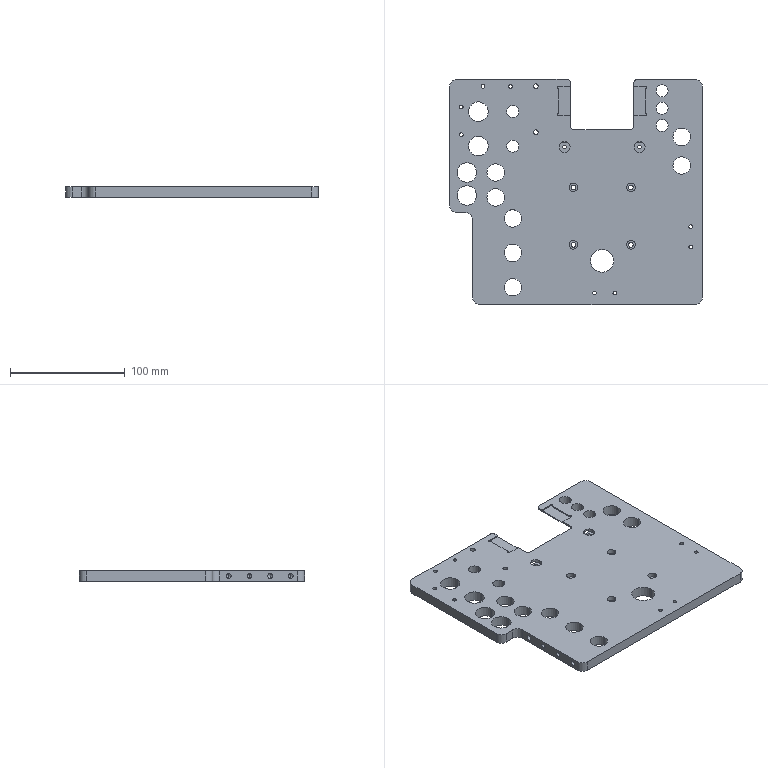NC program | NX | posted with a generic post | part box 220 x 196 x 9 mm
Whole program:
N10 G17 G21 G94 G90
(FLOOR_WALL_COPY_1 , TOOL : D6)
N12 T12 M6
N14 G54
N16 G17 G0 G90 X0.8 Y70.544 S9500 M3
N18 G43 Z30. H12
N20 Z-0.487
N22 G94 G1 X4.5 Y72.68 F2200.
N24 G3 X4.8 Y73.2 R0.6
N26 G1 Y95.
N28 G2 X7.8 Y98. R3.
N30 G1 X21.458
N32 G3 X19.2 Y92. R9.1
N34 G1 Y49.
N36 G2 X16.3 Y46.1 R2.9
N38 G1 X-61.7
N40 G2 X-64.6 Y49. R2.9
N42 G1 Y92.
N44 G3 X-66.858 Y98. R9.1
N46 G1 X-53.25
N48 G2 X-50.25 Y95. R3.
N50 G1 Y54.4
N52 X4.8
N54 Y73.2
N56 X7.8
N58 Y95.
N60 X16.578
N62 G3 X16.2 Y92. R12.1
N64 G1 Y49.1
N66 X-61.6
N68 Y92.
N70 G3 X-61.978 Y95. R12.1
N72 G1 X-53.25
N74 Y54.4
N76 G3 X-53.021 Y53.25 R3.
N78 G1 X-55.792 Y52.1
N80 X-58.6
N82 Y92.
N84 X-56.25
N86 Y54.4
N88 G3 X-55.792 Y52.1 R6.
N90 G1 X-53.021 Y53.25
N92 G3 X-50.25 Y51.4 R3.
N94 G1 X4.8
N96 G3 X7.8 Y54.4 R3.
N98 G1 Y73.2
N100 X10.8
N102 Y92.
N104 X13.2
N106 Y52.1
N108 X10.342
N110 G3 X10.8 Y54.4 R6.
N112 G1 Y73.2
N114 G3 X10.5 Y73.72 R0.6
N116 G0 Z30.
N118 X0.8 Y70.544
N120 Z-0.973
N122 G1 X4.5 Y72.68
N124 G3 X4.8 Y73.2 R0.6
N126 G1 Y95.
N128 G2 X7.8 Y98. R3.
N130 G1 X21.458
N132 G3 X19.2 Y92. R9.1
N134 G1 Y49.
N136 G2 X16.3 Y46.1 R2.9
N138 G1 X-61.7
N140 G2 X-64.6 Y49. R2.9
N142 G1 Y92.
N144 G3 X-66.858 Y98. R9.1
N146 G1 X-53.25
N148 G2 X-50.25 Y95. R3.
N150 G1 Y54.4
N152 X4.8
N154 Y73.2
N156 X7.8
N158 Y95.
N160 X16.578
N162 G3 X16.2 Y92. R12.1
N164 G1 Y49.1
N166 X-61.6
N168 Y92.
N170 G3 X-61.978 Y95. R12.1
N172 G1 X-53.25
N174 Y54.4
N176 G3 X-53.021 Y53.25 R3.
N178 G1 X-55.792 Y52.1
N180 X-58.6
N182 Y92.
N184 X-56.25
N186 Y54.4
N188 G3 X-55.792 Y52.1 R6.
N190 G1 X-53.021 Y53.25
N192 G3 X-50.25 Y51.4 R3.
N194 G1 X4.8
N196 G3 X7.8 Y54.4 R3.
N198 G1 Y73.2
N200 X10.8
N202 Y92.
N204 X13.2
N206 Y52.1
N208 X10.342
N210 G3 X10.8 Y54.4 R6.
N212 G1 Y73.2
N214 G3 X10.5 Y73.72 R0.6
N216 G0 Z30.
N218 X0.8 Y70.544
N220 Z-1.46
N222 G1 X4.5 Y72.68
N224 G3 X4.8 Y73.2 R0.6
N226 G1 Y95.
N228 G2 X7.8 Y98. R3.
N230 G1 X21.458
N232 G3 X19.2 Y92. R9.1
N234 G1 Y49.
N236 G2 X16.3 Y46.1 R2.9
N238 G1 X-61.7
N240 G2 X-64.6 Y49. R2.9
N242 G1 Y92.
N244 G3 X-66.858 Y98. R9.1
N246 G1 X-53.25
N248 G2 X-50.25 Y95. R3.
N250 G1 Y54.4
N252 X4.8
N254 Y73.2
N256 X7.8
N258 Y95.
N260 X16.578
N262 G3 X16.2 Y92. R12.1
N264 G1 Y49.1
N266 X-61.6
N268 Y92.
N270 G3 X-61.978 Y95. R12.1
N272 G1 X-53.25
N274 Y54.4
N276 G3 X-53.021 Y53.25 R3.
N278 G1 X-55.792 Y52.1
N280 X-58.6
N282 Y92.
N284 X-56.25
N286 Y54.4
N288 G3 X-55.792 Y52.1 R6.
N290 G1 X-53.021 Y53.25
N292 G3 X-50.25 Y51.4 R3.
N294 G1 X4.8
N296 G3 X7.8 Y54.4 R3.
N298 G1 Y73.2
N300 X10.8
N302 Y92.
N304 X13.2
N306 Y52.1
N308 X10.342
N310 G3 X10.8 Y54.4 R6.
N312 G1 Y73.2
N314 G3 X10.5 Y73.72 R0.6
N316 G0 Z30.
N318 X0.8 Y70.544
N320 Z-1.947
N322 G1 X4.5 Y72.68
N324 G3 X4.8 Y73.2 R0.6
N326 G1 Y95.
N328 G2 X7.8 Y98. R3.
N330 G1 X21.458
N332 G3 X19.2 Y92. R9.1
N334 G1 Y49.
N336 G2 X16.3 Y46.1 R2.9
N338 G1 X-61.7
N340 G2 X-64.6 Y49. R2.9
N342 G1 Y92.
N344 G3 X-66.858 Y98. R9.1
N346 G1 X-53.25
N348 G2 X-50.25 Y95. R3.
N350 G1 Y54.4
N352 X4.8
N354 Y73.2
N356 X7.8
N358 Y95.
N360 X16.578
N362 G3 X16.2 Y92. R12.1
N364 G1 Y49.1
N366 X-61.6
N368 Y92.
N370 G3 X-61.978 Y95. R12.1
N372 G1 X-53.25
N374 Y54.4
N376 G3 X-53.021 Y53.25 R3.
N378 G1 X-55.792 Y52.1
N380 X-58.6
N382 Y92.
N384 X-56.25
N386 Y54.4
N388 G3 X-55.792 Y52.1 R6.
N390 G1 X-53.021 Y53.25
N392 G3 X-50.25 Y51.4 R3.
N394 G1 X4.8
N396 G3 X7.8 Y54.4 R3.
N398 G1 Y73.2
N400 X10.8
N402 Y92.
N404 X13.2
N406 Y52.1
N408 X10.342
N410 G3 X10.8 Y54.4 R6.
N412 G1 Y73.2
N414 G3 X10.5 Y73.72 R0.6
N416 G0 Z30.
N418 X0.8 Y70.544
N420 Z-2.433
N422 G1 X4.5 Y72.68
N424 G3 X4.8 Y73.2 R0.6
N426 G1 Y95.
N428 G2 X7.8 Y98. R3.
N430 G1 X21.458
N432 G3 X19.2 Y92. R9.1
N434 G1 Y49.
N436 G2 X16.3 Y46.1 R2.9
N438 G1 X-61.7
N440 G2 X-64.6 Y49. R2.9
N442 G1 Y92.
N444 G3 X-66.858 Y98. R9.1
N446 G1 X-53.25
N448 G2 X-50.25 Y95. R3.
N450 G1 Y54.4
N452 X4.8
N454 Y73.2
N456 X7.8
N458 Y95.
N460 X16.578
N462 G3 X16.2 Y92. R12.1
N464 G1 Y49.1
N466 X-61.6
N468 Y92.
N470 G3 X-61.978 Y95. R12.1
N472 G1 X-53.25
N474 Y54.4
N476 G3 X-53.021 Y53.25 R3.
N478 G1 X-55.792 Y52.1
N480 X-58.6
N482 Y92.
N484 X-56.25
N486 Y54.4
N488 G3 X-55.792 Y52.1 R6.
N490 G1 X-53.021 Y53.25
N492 G3 X-50.25 Y51.4 R3.
N494 G1 X4.8
N496 G3 X7.8 Y54.4 R3.
N498 G1 Y73.2
N500 X10.8
N502 Y92.
N504 X13.2
N506 Y52.1
N508 X10.342
N510 G3 X10.8 Y54.4 R6.
N512 G1 Y73.2
N514 G3 X10.5 Y73.72 R0.6
N516 G0 Z30.
N518 X0.8 Y70.544
N520 Z-2.92
N522 G1 X4.5 Y72.68
N524 G3 X4.8 Y73.2 R0.6
N526 G1 Y95.
N528 G2 X7.8 Y98. R3.
N530 G1 X21.458
N532 G3 X19.2 Y92. R9.1
N534 G1 Y49.
N536 G2 X16.3 Y46.1 R2.9
N538 G1 X-61.7
N540 G2 X-64.6 Y49. R2.9
N542 G1 Y92.
N544 G3 X-66.858 Y98. R9.1
N546 G1 X-53.25
N548 G2 X-50.25 Y95. R3.
N550 G1 Y54.4
N552 X4.8
N554 Y73.2
N556 X7.8
N558 Y95.
N560 X16.578
N562 G3 X16.2 Y92. R12.1
N564 G1 Y49.1
N566 X-61.6
N568 Y92.
N570 G3 X-61.978 Y95. R12.1
N572 G1 X-53.25
N574 Y54.4
N576 G3 X-53.021 Y53.25 R3.
N578 G1 X-55.792 Y52.1
N580 X-58.6
N582 Y92.
N584 X-56.25
N586 Y54.4
N588 G3 X-55.792 Y52.1 R6.
N590 G1 X-53.021 Y53.25
N592 G3 X-50.25 Y51.4 R3.
N594 G1 X4.8
N596 G3 X7.8 Y54.4 R3.
N598 G1 Y73.2
N600 X10.8
N602 Y92.
N604 X13.2
N606 Y52.1
N608 X10.342
N610 G3 X10.8 Y54.4 R6.
N612 G1 Y73.2
N614 G3 X10.5 Y73.72 R0.6
N616 G0 Z30.
N618 X0.8 Y70.544
N620 Z-3.407
N622 G1 X4.5 Y72.68
N624 G3 X4.8 Y73.2 R0.6
N626 G1 Y95.
N628 G2 X7.8 Y98. R3.
N630 G1 X21.458
N632 G3 X19.2 Y92. R9.1
N634 G1 Y49.
N636 G2 X16.3 Y46.1 R2.9
N638 G1 X-61.7
N640 G2 X-64.6 Y49. R2.9
N642 G1 Y92.
N644 G3 X-66.858 Y98. R9.1
N646 G1 X-53.25
N648 G2 X-50.25 Y95. R3.
N650 G1 Y54.4
N652 X4.8
N654 Y73.2
N656 X7.8
N658 Y95.
N660 X16.578
N662 G3 X16.2 Y92. R12.1
N664 G1 Y49.1
N666 X-61.6
N668 Y92.
N670 G3 X-61.978 Y95. R12.1
N672 G1 X-53.25
N674 Y54.4
N676 G3 X-53.021 Y53.25 R3.
N678 G1 X-55.792 Y52.1
N680 X-58.6
N682 Y92.
N684 X-56.25
N686 Y54.4
N688 G3 X-55.792 Y52.1 R6.
N690 G1 X-53.021 Y53.25
N692 G3 X-50.25 Y51.4 R3.
N694 G1 X4.8
N696 G3 X7.8 Y54.4 R3.
N698 G1 Y73.2
N700 X10.8
N702 Y92.
N704 X13.2
N706 Y52.1
N708 X10.342
N710 G3 X10.8 Y54.4 R6.
N712 G1 Y73.2
N714 G3 X10.5 Y73.72 R0.6
N716 G0 Z30.
N718 X0.8 Y70.544
N720 Z-3.893
N722 G1 X4.5 Y72.68
N724 G3 X4.8 Y73.2 R0.6
N726 G1 Y95.
N728 G2 X7.8 Y98. R3.
N730 G1 X21.458
N732 G3 X19.2 Y92. R9.1
N734 G1 Y49.
N736 G2 X16.3 Y46.1 R2.9
N738 G1 X-61.7
N740 G2 X-64.6 Y49. R2.9
N742 G1 Y92.
N744 G3 X-66.858 Y98. R9.1
N746 G1 X-53.25
N748 G2 X-50.25 Y95. R3.
N750 G1 Y54.4
N752 X4.8
N754 Y73.2
N756 X7.8
N758 Y95.
N760 X16.578
N762 G3 X16.2 Y92. R12.1
N764 G1 Y49.1
N766 X-61.6
N768 Y92.
N770 G3 X-61.978 Y95. R12.1
N772 G1 X-53.25
N774 Y54.4
N776 G3 X-53.021 Y53.25 R3.
N778 G1 X-55.792 Y52.1
N780 X-58.6
N782 Y92.
N784 X-56.25
N786 Y54.4
N788 G3 X-55.792 Y52.1 R6.
N790 G1 X-53.021 Y53.25
N792 G3 X-50.25 Y51.4 R3.
N794 G1 X4.8
N796 G3 X7.8 Y54.4 R3.
N798 G1 Y73.2
N800 X10.8
N802 Y92.
N804 X13.2
N806 Y52.1
N808 X10.342
N810 G3 X10.8 Y54.4 R6.
N812 G1 Y73.2
N814 G3 X10.5 Y73.72 R0.6
N816 G0 Z30.
N818 X0.8 Y70.544
N820 Z-4.38
N822 G1 X4.5 Y72.68
N824 G3 X4.8 Y73.2 R0.6
N826 G1 Y95.
N828 G2 X7.8 Y98. R3.
N830 G1 X21.458
N832 G3 X19.2 Y92. R9.1
N834 G1 Y49.
N836 G2 X16.3 Y46.1 R2.9
N838 G1 X-61.7
N840 G2 X-64.6 Y49. R2.9
N842 G1 Y92.
N844 G3 X-66.858 Y98. R9.1
N846 G1 X-53.25
N848 G2 X-50.25 Y95. R3.
N850 G1 Y54.4
N852 X4.8
N854 Y73.2
N856 X7.8
N858 Y95.
N860 X16.578
N862 G3 X16.2 Y92. R12.1
N864 G1 Y49.1
N866 X-61.6
N868 Y92.
N870 G3 X-61.978 Y95. R12.1
N872 G1 X-53.25
N874 Y54.4
N876 G3 X-53.021 Y53.25 R3.
N878 G1 X-55.792 Y52.1
N880 X-58.6
N882 Y92.
N884 X-56.25
N886 Y54.4
N888 G3 X-55.792 Y52.1 R6.
N890 G1 X-53.021 Y53.25
N892 G3 X-50.25 Y51.4 R3.
N894 G1 X4.8
N896 G3 X7.8 Y54.4 R3.
N898 G1 Y73.2
N900 X10.8
N902 Y92.
N904 X13.2
N906 Y52.1
N908 X10.342
N910 G3 X10.8 Y54.4 R6.
N912 G1 Y73.2
N914 G3 X10.5 Y73.72 R0.6
N916 G0 Z30.
N918 X0.8 Y70.544
N920 Z-4.867
N922 G1 X4.5 Y72.68
N924 G3 X4.8 Y73.2 R0.6
N926 G1 Y95.
N928 G2 X7.8 Y98. R3.
N930 G1 X21.458
N932 G3 X19.2 Y92. R9.1
N934 G1 Y49.
N936 G2 X16.3 Y46.1 R2.9
N938 G1 X-61.7
N940 G2 X-64.6 Y49. R2.9
N942 G1 Y92.
N944 G3 X-66.858 Y98. R9.1
N946 G1 X-53.25
N948 G2 X-50.25 Y95. R3.
N950 G1 Y54.4
N952 X4.8
N954 Y73.2
N956 X7.8
N958 Y95.
N960 X16.578
N962 G3 X16.2 Y92. R12.1
N964 G1 Y49.1
N966 X-61.6
N968 Y92.
N970 G3 X-61.978 Y95. R12.1
N972 G1 X-53.25
N974 Y54.4
N976 G3 X-53.021 Y53.25 R3.
N978 G1 X-55.792 Y52.1
N980 X-58.6
N982 Y92.
N984 X-56.25
N986 Y54.4
N988 G3 X-55.792 Y52.1 R6.
N990 G1 X-53.021 Y53.25
N992 G3 X-50.25 Y51.4 R3.
N994 G1 X4.8
N996 G3 X7.8 Y54.4 R3.
N998 G1 Y73.2
N1000 X10.8
N1002 Y92.
N1004 X13.2
N1006 Y52.1
N1008 X10.342
N1010 G3 X10.8 Y54.4 R6.
N1012 G1 Y73.2
N1014 G3 X10.5 Y73.72 R0.6
N1016 G0 Z30.
N1018 X0.8 Y70.544
N1020 Z-5.353
N1022 G1 X4.5 Y72.68
N1024 G3 X4.8 Y73.2 R0.6
N1026 G1 Y95.
N1028 G2 X7.8 Y98. R3.
N1030 G1 X21.458
N1032 G3 X19.2 Y92. R9.1
N1034 G1 Y49.
N1036 G2 X16.3 Y46.1 R2.9
N1038 G1 X-61.7
N1040 G2 X-64.6 Y49. R2.9
N1042 G1 Y92.
N1044 G3 X-66.858 Y98. R9.1
N1046 G1 X-53.25
N1048 G2 X-50.25 Y95. R3.
N1050 G1 Y54.4
N1052 X4.8
N1054 Y73.2
N1056 X7.8
N1058 Y95.
N1060 X16.578
N1062 G3 X16.2 Y92. R12.1
N1064 G1 Y49.1
N1066 X-61.6
N1068 Y92.
N1070 G3 X-61.978 Y95. R12.1
N1072 G1 X-53.25
N1074 Y54.4
N1076 G3 X-53.021 Y53.25 R3.
N1078 G1 X-55.792 Y52.1
N1080 X-58.6
N1082 Y92.
N1084 X-56.25
N1086 Y54.4
N1088 G3 X-55.792 Y52.1 R6.
N1090 G1 X-53.021 Y53.25
N1092 G3 X-50.25 Y51.4 R3.
N1094 G1 X4.8
N1096 G3 X7.8 Y54.4 R3.
N1098 G1 Y73.2
N1100 X10.8
N1102 Y92.
N1104 X13.2
N1106 Y52.1
N1108 X10.342
N1110 G3 X10.8 Y54.4 R6.
N1112 G1 Y73.2
N1114 G3 X10.5 Y73.72 R0.6
N1116 G0 Z30.
N1118 X0.8 Y70.544
N1120 Z-5.84
N1122 G1 X4.5 Y72.68
N1124 G3 X4.8 Y73.2 R0.6
N1126 G1 Y95.
N1128 G2 X7.8 Y98. R3.
N1130 G1 X21.458
N1132 G3 X19.2 Y92. R9.1
N1134 G1 Y49.
N1136 G2 X16.3 Y46.1 R2.9
N1138 G1 X-61.7
N1140 G2 X-64.6 Y49. R2.9
N1142 G1 Y92.
N1144 G3 X-66.858 Y98. R9.1
N1146 G1 X-53.25
N1148 G2 X-50.25 Y95. R3.
N1150 G1 Y54.4
N1152 X4.8
N1154 Y73.2
N1156 X7.8
N1158 Y95.
N1160 X16.578
N1162 G3 X16.2 Y92. R12.1
N1164 G1 Y49.1
N1166 X-61.6
N1168 Y92.
N1170 G3 X-61.978 Y95. R12.1
N1172 G1 X-53.25
N1174 Y54.4
N1176 G3 X-53.021 Y53.25 R3.
N1178 G1 X-55.792 Y52.1
N1180 X-58.6
N1182 Y92.
N1184 X-56.25
N1186 Y54.4
N1188 G3 X-55.792 Y52.1 R6.
N1190 G1 X-53.021 Y53.25
N1192 G3 X-50.25 Y51.4 R3.
N1194 G1 X4.8
N1196 G3 X7.8 Y54.4 R3.
N1198 G1 Y73.2
N1200 X10.8
N1202 Y92.
N1204 X13.2
N1206 Y52.1
N1208 X10.342
N1210 G3 X10.8 Y54.4 R6.
N1212 G1 Y73.2
N1214 G3 X10.5 Y73.72 R0.6
N1216 G0 Z30.
N1218 X0.8 Y70.544
N1220 Z-6.327
N1222 G1 X4.5 Y72.68
N1224 G3 X4.8 Y73.2 R0.6
N1226 G1 Y95.
N1228 G2 X7.8 Y98. R3.
N1230 G1 X21.458
N1232 G3 X19.2 Y92. R9.1
N1234 G1 Y49.
N1236 G2 X16.3 Y46.1 R2.9
N1238 G1 X-61.7
N1240 G2 X-64.6 Y49. R2.9
N1242 G1 Y92.
N1244 G3 X-66.858 Y98. R9.1
N1246 G1 X-53.25
N1248 G2 X-50.25 Y95. R3.
N1250 G1 Y54.4
N1252 X4.8
N1254 Y73.2
N1256 X7.8
N1258 Y95.
N1260 X16.578
N1262 G3 X16.2 Y92. R12.1
N1264 G1 Y49.1
N1266 X-61.6
N1268 Y92.
N1270 G3 X-61.978 Y95. R12.1
N1272 G1 X-53.25
N1274 Y54.4
N1276 G3 X-53.021 Y53.25 R3.
N1278 G1 X-55.792 Y52.1
N1280 X-58.6
N1282 Y92.
N1284 X-56.25
N1286 Y54.4
N1288 G3 X-55.792 Y52.1 R6.
N1290 G1 X-53.021 Y53.25
N1292 G3 X-50.25 Y51.4 R3.
N1294 G1 X4.8
N1296 G3 X7.8 Y54.4 R3.
N1298 G1 Y73.2
N1300 X10.8
N1302 Y92.
N1304 X13.2
N1306 Y52.1
N1308 X10.342
N1310 G3 X10.8 Y54.4 R6.
N1312 G1 Y73.2
N1314 G3 X10.5 Y73.72 R0.6
N1316 G0 Z30.
N1318 X0.8 Y70.544
N1320 Z-6.813
N1322 G1 X4.5 Y72.68
N1324 G3 X4.8 Y73.2 R0.6
N1326 G1 Y95.
N1328 G2 X7.8 Y98. R3.
N1330 G1 X21.458
N1332 G3 X19.2 Y92. R9.1
N1334 G1 Y49.
N1336 G2 X16.3 Y46.1 R2.9
N1338 G1 X-61.7
N1340 G2 X-64.6 Y49. R2.9
N1342 G1 Y92.
N1344 G3 X-66.858 Y98. R9.1
N1346 G1 X-53.25
N1348 G2 X-50.25 Y95. R3.
N1350 G1 Y54.4
N1352 X4.8
N1354 Y73.2
N1356 X7.8
N1358 Y95.
N1360 X16.578
N1362 G3 X16.2 Y92. R12.1
N1364 G1 Y49.1
N1366 X-61.6
N1368 Y92.
N1370 G3 X-61.978 Y95. R12.1
N1372 G1 X-53.25
N1374 Y54.4
N1376 G3 X-53.021 Y53.25 R3.
N1378 G1 X-55.792 Y52.1
N1380 X-58.6
N1382 Y92.
N1384 X-56.25
N1386 Y54.4
N1388 G3 X-55.792 Y52.1 R6.
N1390 G1 X-53.021 Y53.25
N1392 G3 X-50.25 Y51.4 R3.
N1394 G1 X4.8
N1396 G3 X7.8 Y54.4 R3.
N1398 G1 Y73.2
N1400 X10.8
N1402 Y92.
N1404 X13.2
N1406 Y52.1
N1408 X10.342
N1410 G3 X10.8 Y54.4 R6.
N1412 G1 Y73.2
N1414 G3 X10.5 Y73.72 R0.6
N1416 G0 Z30.
N1418 X0.8 Y70.544
N1420 Z-7.3
N1422 G1 X4.5 Y72.68
N1424 G3 X4.8 Y73.2 R0.6
N1426 G1 Y95.
N1428 G2 X7.8 Y98. R3.
N1430 G1 X21.458
N1432 G3 X19.2 Y92. R9.1
N1434 G1 Y49.
N1436 G2 X16.3 Y46.1 R2.9
N1438 G1 X-61.7
N1440 G2 X-64.6 Y49. R2.9
N1442 G1 Y92.
N1444 G3 X-66.858 Y98. R9.1
N1446 G1 X-53.25
N1448 G2 X-50.25 Y95. R3.
N1450 G1 Y54.4
N1452 X4.8
N1454 Y73.2
N1456 X7.8
N1458 Y95.
N1460 X16.578
N1462 G3 X16.2 Y92. R12.1
N1464 G1 Y49.1
N1466 X-61.6
N1468 Y92.
N1470 G3 X-61.978 Y95. R12.1
N1472 G1 X-53.25
N1474 Y54.4
N1476 G3 X-53.021 Y53.25 R3.
N1478 G1 X-55.792 Y52.1
N1480 X-58.6
N1482 Y92.
N1484 X-56.25
N1486 Y54.4
N1488 G3 X-55.792 Y52.1 R6.
N1490 G1 X-53.021 Y53.25
N1492 G3 X-50.25 Y51.4 R3.
N1494 G1 X4.8
N1496 G3 X7.8 Y54.4 R3.
N1498 G1 Y73.2
N1500 X10.8
N1502 Y92.
N1504 X13.2
N1506 Y52.1
N1508 X10.342
N1510 G3 X10.8 Y54.4 R6.
N1512 G1 Y73.2
N1514 G3 X10.5 Y73.72 R0.6
N1516 G0 Z30.
(FLOOR_WALL_1 , TOOL : D6)
N1518 X-1.2 Y60.4
N1520 Z-4.4
N1522 G1 Z-7.4 F1250.
N1524 Y57.4
N1526 X1.8
N1528 Y95.
N1530 G2 X7.8 Y101. R6.
N1532 G1 X25.957
N1534 G3 X19. Y92. R9.3
N1536 G1 Y49.
N1538 G2 X16.3 Y46.3 R2.7
N1540 G1 X-61.7
N1542 G2 X-64.4 Y49. R2.7
N1544 G1 Y92.
N1546 G3 X-71.357 Y101. R9.3
N1548 G1 X-53.25
N1550 G2 X-47.25 Y95. R6.
N1552 G1 Y57.4
N1554 X1.8
N1556 X3.745 Y55.116
N1558 G3 X4.8 Y57.4 R3.
N1560 G1 Y95.
N1562 G2 X7.8 Y98. R3.
N1564 G1 X17.563
N1566 G3 X16. Y92. R12.3
N1568 G1 Y49.3
N1570 X-61.4
N1572 Y92.
N1574 G3 X-62.963 Y98. R12.3
N1576 G1 X-53.25
N1578 G2 X-50.25 Y95. R3.
N1580 G1 Y57.4
N1582 G3 X-48.83 Y54.85 R3.
N1584 G1 X-50.411 Y52.3
N1586 X-58.4
N1588 Y92.
N1590 G3 X-58.697 Y95. R15.3
N1592 G1 X-53.25
N1594 Y57.4
N1596 G3 X-50.411 Y52.3 R6.
N1598 G1 X-55.612 Y55.
N1600 X-55.7
N1602 Y55.329
N1604 G3 X-55.612 Y55. R8.7
N1606 G1 X-50.411 Y52.3
N1608 X-48.83 Y54.85
N1610 G3 X-47.25 Y54.4 R3.
N1612 G1 X1.8
N1614 G3 X3.745 Y55.116 R3.
N1616 G1 X5.69 Y52.832
N1618 G3 X7.8 Y57.4 R6.
N1620 G1 Y95.
N1622 X13.297
N1624 G3 X13. Y92. R15.3
N1626 G1 Y52.3
N1628 X4.961
N1630 G3 X5.69 Y52.832 R6.
N1632 G1 X10.162 Y55.
N1634 G3 X10.3 Y55.545 R8.7
N1636 G1 Y55.
N1638 X10.162
N1640 Y52.
N1642 Z-4.4
N1644 G0 Z30.
N1646 X-75.956 Y104.
N1648 Z-4.4
N1650 G1 Z-7.4
N1652 Y101.215
N1654 X-72.966 Y100.97
N1656 G2 X-64.7 Y92. R9.
N1658 G1 Y49.
N1660 G3 X-61.7 Y46. R3.
N1662 G1 X16.3
N1664 G3 X19.3 Y49. R3.
N1666 G1 Y92.
N1668 G2 X27.566 Y100.97 R9.
N1670 G1 X30.556 Y101.215
N1672 Y104.
N1674 Z-4.4
N1676 G0 Z30.
(HOLE_MILLING_COPY , TOOL : D6)
N1678 X35. Y92.
N1680 Z0.5
N1682 G3 X34.625 Y92.375 R0.375
N1684 X34.25 Y92. R0.375
N1686 X34.25 Y92. Z0. I0.75 J0.
N1688 X34.25 Y92. Z-0.5 I0.75 J0.
N1690 X34.25 Y92. Z-1. I0.75 J0.
N1692 X34.25 Y92. Z-1.5 I0.75 J0.
N1694 X34.25 Y92. Z-2. I0.75 J0.
N1696 X34.25 Y92. Z-2.5 I0.75 J0.
N1698 X34.25 Y92. Z-3. I0.75 J0.
N1700 X34.25 Y92. Z-3.5 I0.75 J0.
N1702 X34.25 Y92. Z-4. I0.75 J0.
N1704 X35. Y91.25 R0.75
N1706 X34.25 Y92. R-0.75
N1708 X34.625 Y91.625 R0.375
N1710 X35. Y92. R0.375
N1712 G0 Z30.
N1714 Y52.
N1716 Z0.5
N1718 G3 X34.625 Y52.375 R0.375
N1720 X34.25 Y52. R0.375
N1722 X34.25 Y52. Z0. I0.75 J0.
N1724 X34.25 Y52. Z-0.5 I0.75 J0.
N1726 X34.25 Y52. Z-1. I0.75 J0.
N1728 X34.25 Y52. Z-1.5 I0.75 J0.
N1730 X34.25 Y52. Z-2. I0.75 J0.
N1732 X34.25 Y52. Z-2.5 I0.75 J0.
N1734 X34.25 Y52. Z-3. I0.75 J0.
N1736 X34.25 Y52. Z-3.5 I0.75 J0.
N1738 X34.25 Y52. Z-4. I0.75 J0.
N1740 X35. Y51.25 R0.75
N1742 X34.25 Y52. R-0.75
N1744 X34.625 Y51.625 R0.375
N1746 X35. Y52. R0.375
N1748 G0 Z30.
N1750 M5
(HOLE_MILLING_1 , TOOL : D3)
N1752 T18 M6
N1754 G54
N1756 G17 G0 G90 X-103. Y-68. S9500 M3
N1758 G43 Z30. H18
N1760 Z1.
N1762 G94 G3 X-103.3 Y-67.7 R0.3 F1250.
N1764 X-103.6 Y-68. R0.3
N1766 X-103.6 Y-68. Z0.8 I0.6 J0.
N1768 X-103.6 Y-68. Z0.6 I0.6 J0.
N1770 X-103.6 Y-68. Z0.4 I0.6 J0.
N1772 X-103.6 Y-68. Z0.2 I0.6 J0.
N1774 X-103.6 Y-68. Z0. I0.6 J0.
N1776 X-103.6 Y-68. Z-0.2 I0.6 J0.
N1778 X-103.6 Y-68. Z-0.4 I0.6 J0.
N1780 X-103.6 Y-68. Z-0.6 I0.6 J0.
N1782 X-103.6 Y-68. Z-0.8 I0.6 J0.
N1784 X-103.6 Y-68. Z-1. I0.6 J0.
N1786 X-103.6 Y-68. Z-1.2 I0.6 J0.
N1788 X-103.6 Y-68. Z-1.4 I0.6 J0.
N1790 X-103.6 Y-68. Z-1.6 I0.6 J0.
N1792 X-103.6 Y-68. Z-1.8 I0.6 J0.
N1794 X-103.6 Y-68. Z-2. I0.6 J0.
N1796 X-103.6 Y-68. Z-2.2 I0.6 J0.
N1798 X-103.6 Y-68. Z-2.4 I0.6 J0.
N1800 X-103.6 Y-68. Z-2.6 I0.6 J0.
N1802 X-103.6 Y-68. Z-2.8 I0.6 J0.
N1804 X-103.6 Y-68. Z-3. I0.6 J0.
N1806 X-103.6 Y-68. Z-3.2 I0.6 J0.
N1808 X-103.6 Y-68. Z-3.4 I0.6 J0.
N1810 X-103.6 Y-68. Z-3.6 I0.6 J0.
N1812 X-103.6 Y-68. Z-3.8 I0.6 J0.
N1814 X-103.6 Y-68. Z-4. I0.6 J0.
N1816 X-103.6 Y-68. Z-4.2 I0.6 J0.
N1818 X-103.6 Y-68. Z-4.4 I0.6 J0.
N1820 X-103.6 Y-68. Z-4.6 I0.6 J0.
N1822 X-103.6 Y-68. Z-4.8 I0.6 J0.
N1824 X-103.6 Y-68. Z-5. I0.6 J0.
N1826 X-103.6 Y-68. Z-5.2 I0.6 J0.
N1828 X-103.6 Y-68. Z-5.4 I0.6 J0.
N1830 X-103.6 Y-68. Z-5.6 I0.6 J0.
N1832 X-103.6 Y-68. Z-5.8 I0.6 J0.
N1834 X-103.6 Y-68. Z-6. I0.6 J0.
N1836 X-103. Y-68.6 R0.6
N1838 X-103.6 Y-68. R-0.6
N1840 X-103.3 Y-68.3 R0.3
N1842 X-103. Y-68. R0.3
N1844 G0 Z30.
N1846 Y-86.
N1848 Z1.
N1850 G3 X-103.3 Y-85.7 R0.3
N1852 X-103.6 Y-86. R0.3
N1854 X-103.6 Y-86. Z0.8 I0.6 J0.
N1856 X-103.6 Y-86. Z0.6 I0.6 J0.
N1858 X-103.6 Y-86. Z0.4 I0.6 J0.
N1860 X-103.6 Y-86. Z0.2 I0.6 J0.
N1862 X-103.6 Y-86. Z0. I0.6 J0.
N1864 X-103.6 Y-86. Z-0.2 I0.6 J0.
N1866 X-103.6 Y-86. Z-0.4 I0.6 J0.
N1868 X-103.6 Y-86. Z-0.6 I0.6 J0.
N1870 X-103.6 Y-86. Z-0.8 I0.6 J0.
N1872 X-103.6 Y-86. Z-1. I0.6 J0.
N1874 X-103.6 Y-86. Z-1.2 I0.6 J0.
N1876 X-103.6 Y-86. Z-1.4 I0.6 J0.
N1878 X-103.6 Y-86. Z-1.6 I0.6 J0.
N1880 X-103.6 Y-86. Z-1.8 I0.6 J0.
N1882 X-103.6 Y-86. Z-2. I0.6 J0.
N1884 X-103.6 Y-86. Z-2.2 I0.6 J0.
N1886 X-103.6 Y-86. Z-2.4 I0.6 J0.
N1888 X-103.6 Y-86. Z-2.6 I0.6 J0.
N1890 X-103.6 Y-86. Z-2.8 I0.6 J0.
N1892 X-103.6 Y-86. Z-3. I0.6 J0.
N1894 X-103.6 Y-86. Z-3.2 I0.6 J0.
N1896 X-103.6 Y-86. Z-3.4 I0.6 J0.
N1898 X-103.6 Y-86. Z-3.6 I0.6 J0.
N1900 X-103.6 Y-86. Z-3.8 I0.6 J0.
N1902 X-103.6 Y-86. Z-4. I0.6 J0.
N1904 X-103.6 Y-86. Z-4.2 I0.6 J0.
N1906 X-103.6 Y-86. Z-4.4 I0.6 J0.
N1908 X-103.6 Y-86. Z-4.6 I0.6 J0.
N1910 X-103.6 Y-86. Z-4.8 I0.6 J0.
N1912 X-103.6 Y-86. Z-5. I0.6 J0.
N1914 X-103.6 Y-86. Z-5.2 I0.6 J0.
N1916 X-103.6 Y-86. Z-5.4 I0.6 J0.
N1918 X-103.6 Y-86. Z-5.6 I0.6 J0.
N1920 X-103.6 Y-86. Z-5.8 I0.6 J0.
N1922 X-103.6 Y-86. Z-6. I0.6 J0.
N1924 X-103. Y-86.6 R0.6
N1926 X-103.6 Y-86. R-0.6
N1928 X-103.3 Y-86.3 R0.3
N1930 X-103. Y-86. R0.3
N1932 G0 Z30.
N1934 X83.
N1936 Z1.
N1938 G3 X82.7 Y-85.7 R0.3
N1940 X82.4 Y-86. R0.3
N1942 X82.4 Y-86. Z0.8 I0.6 J0.
N1944 X82.4 Y-86. Z0.6 I0.6 J0.
N1946 X82.4 Y-86. Z0.4 I0.6 J0.
N1948 X82.4 Y-86. Z0.2 I0.6 J0.
N1950 X82.4 Y-86. Z0. I0.6 J0.
N1952 X82.4 Y-86. Z-0.2 I0.6 J0.
N1954 X82.4 Y-86. Z-0.4 I0.6 J0.
N1956 X82.4 Y-86. Z-0.6 I0.6 J0.
N1958 X82.4 Y-86. Z-0.8 I0.6 J0.
N1960 X82.4 Y-86. Z-1. I0.6 J0.
N1962 X82.4 Y-86. Z-1.2 I0.6 J0.
N1964 X82.4 Y-86. Z-1.4 I0.6 J0.
N1966 X82.4 Y-86. Z-1.6 I0.6 J0.
N1968 X82.4 Y-86. Z-1.8 I0.6 J0.
N1970 X82.4 Y-86. Z-2. I0.6 J0.
N1972 X82.4 Y-86. Z-2.2 I0.6 J0.
N1974 X82.4 Y-86. Z-2.4 I0.6 J0.
N1976 X82.4 Y-86. Z-2.6 I0.6 J0.
N1978 X82.4 Y-86. Z-2.8 I0.6 J0.
N1980 X82.4 Y-86. Z-3. I0.6 J0.
N1982 X82.4 Y-86. Z-3.2 I0.6 J0.
N1984 X82.4 Y-86. Z-3.4 I0.6 J0.
N1986 X82.4 Y-86. Z-3.6 I0.6 J0.
N1988 X82.4 Y-86. Z-3.8 I0.6 J0.
N1990 X82.4 Y-86. Z-4. I0.6 J0.
N1992 X82.4 Y-86. Z-4.2 I0.6 J0.
N1994 X82.4 Y-86. Z-4.4 I0.6 J0.
N1996 X82.4 Y-86. Z-4.6 I0.6 J0.
N1998 X82.4 Y-86. Z-4.8 I0.6 J0.
N2000 X82.4 Y-86. Z-5. I0.6 J0.
N2002 X82.4 Y-86. Z-5.2 I0.6 J0.
N2004 X82.4 Y-86. Z-5.4 I0.6 J0.
N2006 X82.4 Y-86. Z-5.6 I0.6 J0.
N2008 X82.4 Y-86. Z-5.8 I0.6 J0.
N2010 X82.4 Y-86. Z-6. I0.6 J0.
N2012 X83. Y-86.6 R0.6
N2014 X82.4 Y-86. R-0.6
N2016 X82.7 Y-86.3 R0.3
N2018 X83. Y-86. R0.3
N2020 G0 Z30.
N2022 Y-68.
N2024 Z1.
N2026 G3 X82.7 Y-67.7 R0.3
N2028 X82.4 Y-68. R0.3
N2030 X82.4 Y-68. Z0.8 I0.6 J0.
N2032 X82.4 Y-68. Z0.6 I0.6 J0.
N2034 X82.4 Y-68. Z0.4 I0.6 J0.
N2036 X82.4 Y-68. Z0.2 I0.6 J0.
N2038 X82.4 Y-68. Z0. I0.6 J0.
N2040 X82.4 Y-68. Z-0.2 I0.6 J0.
N2042 X82.4 Y-68. Z-0.4 I0.6 J0.
N2044 X82.4 Y-68. Z-0.6 I0.6 J0.
N2046 X82.4 Y-68. Z-0.8 I0.6 J0.
N2048 X82.4 Y-68. Z-1. I0.6 J0.
N2050 X82.4 Y-68. Z-1.2 I0.6 J0.
N2052 X82.4 Y-68. Z-1.4 I0.6 J0.
N2054 X82.4 Y-68. Z-1.6 I0.6 J0.
N2056 X82.4 Y-68. Z-1.8 I0.6 J0.
N2058 X82.4 Y-68. Z-2. I0.6 J0.
N2060 X82.4 Y-68. Z-2.2 I0.6 J0.
N2062 X82.4 Y-68. Z-2.4 I0.6 J0.
N2064 X82.4 Y-68. Z-2.6 I0.6 J0.
N2066 X82.4 Y-68. Z-2.8 I0.6 J0.
N2068 X82.4 Y-68. Z-3. I0.6 J0.
N2070 X82.4 Y-68. Z-3.2 I0.6 J0.
N2072 X82.4 Y-68. Z-3.4 I0.6 J0.
N2074 X82.4 Y-68. Z-3.6 I0.6 J0.
N2076 X82.4 Y-68. Z-3.8 I0.6 J0.
N2078 X82.4 Y-68. Z-4. I0.6 J0.
N2080 X82.4 Y-68. Z-4.2 I0.6 J0.
N2082 X82.4 Y-68. Z-4.4 I0.6 J0.
N2084 X82.4 Y-68. Z-4.6 I0.6 J0.
N2086 X82.4 Y-68. Z-4.8 I0.6 J0.
N2088 X82.4 Y-68. Z-5. I0.6 J0.
N2090 X82.4 Y-68. Z-5.2 I0.6 J0.
N2092 X82.4 Y-68. Z-5.4 I0.6 J0.
N2094 X82.4 Y-68. Z-5.6 I0.6 J0.
N2096 X82.4 Y-68. Z-5.8 I0.6 J0.
N2098 X82.4 Y-68. Z-6. I0.6 J0.
N2100 X83. Y-68.6 R0.6
N2102 X82.4 Y-68. R-0.6
N2104 X82.7 Y-68.3 R0.3
N2106 X83. Y-68. R0.3
N2108 G0 Z30.
N2110 Y-50.
N2112 Z1.
N2114 G3 X82.7 Y-49.7 R0.3
N2116 X82.4 Y-50. R0.3
N2118 X82.4 Y-50. Z0.8 I0.6 J0.
N2120 X82.4 Y-50. Z0.6 I0.6 J0.
N2122 X82.4 Y-50. Z0.4 I0.6 J0.
N2124 X82.4 Y-50. Z0.2 I0.6 J0.
N2126 X82.4 Y-50. Z0. I0.6 J0.
N2128 X82.4 Y-50. Z-0.2 I0.6 J0.
N2130 X82.4 Y-50. Z-0.4 I0.6 J0.
N2132 X82.4 Y-50. Z-0.6 I0.6 J0.
N2134 X82.4 Y-50. Z-0.8 I0.6 J0.
N2136 X82.4 Y-50. Z-1. I0.6 J0.
N2138 X82.4 Y-50. Z-1.2 I0.6 J0.
N2140 X82.4 Y-50. Z-1.4 I0.6 J0.
N2142 X82.4 Y-50. Z-1.6 I0.6 J0.
N2144 X82.4 Y-50. Z-1.8 I0.6 J0.
N2146 X82.4 Y-50. Z-2. I0.6 J0.
N2148 X82.4 Y-50. Z-2.2 I0.6 J0.
N2150 X82.4 Y-50. Z-2.4 I0.6 J0.
N2152 X82.4 Y-50. Z-2.6 I0.6 J0.
N2154 X82.4 Y-50. Z-2.8 I0.6 J0.
N2156 X82.4 Y-50. Z-3. I0.6 J0.
N2158 X82.4 Y-50. Z-3.2 I0.6 J0.
N2160 X82.4 Y-50. Z-3.4 I0.6 J0.
N2162 X82.4 Y-50. Z-3.6 I0.6 J0.
N2164 X82.4 Y-50. Z-3.8 I0.6 J0.
N2166 X82.4 Y-50. Z-4. I0.6 J0.
N2168 X82.4 Y-50. Z-4.2 I0.6 J0.
N2170 X82.4 Y-50. Z-4.4 I0.6 J0.
N2172 X82.4 Y-50. Z-4.6 I0.6 J0.
N2174 X82.4 Y-50. Z-4.8 I0.6 J0.
N2176 X82.4 Y-50. Z-5. I0.6 J0.
N2178 X82.4 Y-50. Z-5.2 I0.6 J0.
N2180 X82.4 Y-50. Z-5.4 I0.6 J0.
N2182 X82.4 Y-50. Z-5.6 I0.6 J0.
N2184 X82.4 Y-50. Z-5.8 I0.6 J0.
N2186 X82.4 Y-50. Z-6. I0.6 J0.
N2188 X83. Y-50.6 R0.6
N2190 X82.4 Y-50. R-0.6
N2192 X82.7 Y-50.3 R0.3
N2194 X83. Y-50. R0.3
N2196 G0 Z30.
N2198 Y-32.
N2200 Z1.
N2202 G3 X82.7 Y-31.7 R0.3
N2204 X82.4 Y-32. R0.3
N2206 X82.4 Y-32. Z0.8 I0.6 J0.
N2208 X82.4 Y-32. Z0.6 I0.6 J0.
N2210 X82.4 Y-32. Z0.4 I0.6 J0.
N2212 X82.4 Y-32. Z0.2 I0.6 J0.
N2214 X82.4 Y-32. Z0. I0.6 J0.
N2216 X82.4 Y-32. Z-0.2 I0.6 J0.
N2218 X82.4 Y-32. Z-0.4 I0.6 J0.
N2220 X82.4 Y-32. Z-0.6 I0.6 J0.
N2222 X82.4 Y-32. Z-0.8 I0.6 J0.
N2224 X82.4 Y-32. Z-1. I0.6 J0.
N2226 X82.4 Y-32. Z-1.2 I0.6 J0.
N2228 X82.4 Y-32. Z-1.4 I0.6 J0.
N2230 X82.4 Y-32. Z-1.6 I0.6 J0.
N2232 X82.4 Y-32. Z-1.8 I0.6 J0.
N2234 X82.4 Y-32. Z-2. I0.6 J0.
N2236 X82.4 Y-32. Z-2.2 I0.6 J0.
N2238 X82.4 Y-32. Z-2.4 I0.6 J0.
N2240 X82.4 Y-32. Z-2.6 I0.6 J0.
N2242 X82.4 Y-32. Z-2.8 I0.6 J0.
N2244 X82.4 Y-32. Z-3. I0.6 J0.
N2246 X82.4 Y-32. Z-3.2 I0.6 J0.
N2248 X82.4 Y-32. Z-3.4 I0.6 J0.
N2250 X82.4 Y-32. Z-3.6 I0.6 J0.
N2252 X82.4 Y-32. Z-3.8 I0.6 J0.
N2254 X82.4 Y-32. Z-4. I0.6 J0.
N2256 X82.4 Y-32. Z-4.2 I0.6 J0.
N2258 X82.4 Y-32. Z-4.4 I0.6 J0.
N2260 X82.4 Y-32. Z-4.6 I0.6 J0.
N2262 X82.4 Y-32. Z-4.8 I0.6 J0.
N2264 X82.4 Y-32. Z-5. I0.6 J0.
N2266 X82.4 Y-32. Z-5.2 I0.6 J0.
N2268 X82.4 Y-32. Z-5.4 I0.6 J0.
N2270 X82.4 Y-32. Z-5.6 I0.6 J0.
N2272 X82.4 Y-32. Z-5.8 I0.6 J0.
N2274 X82.4 Y-32. Z-6. I0.6 J0.
N2276 X83. Y-32.6 R0.6
N2278 X82.4 Y-32. R-0.6
N2280 X82.7 Y-32.3 R0.3
N2282 X83. Y-32. R0.3
N2284 G0 Z30.
N2286 M5
(PLANAR_MILL_COPY_COPY_COPY_COPY_COPY_COPY_1_COPY_1_COPY , TOOL : D6A45)
N2288 T01 M6
N2290 G54
N2292 G17 G0 G90 X-103.95 Y-85.134 S9500 M3
N2294 G43 Z30. H1
N2296 Z0.65
N2298 G94 G1 Z-0.85 F1250.
N2300 G3 X-104.45 Y-86. R1.
N2302 X-103. Y-87.45 R1.45
N2304 X-104.45 Y-86. R-1.45
N2306 X-103.95 Y-86.866 R1.
N2308 G1 Z0.65
N2310 G0 Z30.
N2312 Y-67.134
N2314 Z0.65
N2316 G1 Z-0.85
N2318 G3 X-104.45 Y-68. R1.
N2320 X-103. Y-69.45 R1.45
N2322 X-104.45 Y-68. R-1.45
N2324 X-103.95 Y-68.866 R1.
N2326 G1 Z0.65
N2328 G0 Z30.
N2330 X-100.5 Y-47.134
N2332 Z0.65
N2334 G1 Z-0.85
N2336 G3 X-101. Y-48. R1.
N2338 X-100. Y-49. R1.
N2340 X-101. Y-48. R-1.
N2342 X-100.5 Y-48.866 R1.
N2344 G1 Z0.65
N2346 G0 Z30.
N2348 Y-29.334
N2350 Z0.65
N2352 G1 Z-0.85
N2354 G3 X-101. Y-30.2 R1.
N2356 X-100. Y-31.2 R1.
N2358 X-101. Y-30.2 R-1.
N2360 X-100.5 Y-31.066 R1.
N2362 G1 Z0.65
N2364 G0 Z30.
N2366 X-98.45 Y23.866
N2368 Z0.65
N2370 G1 Z-0.85
N2372 G3 X-98.95 Y23. R1.
N2374 X-92. Y16.05 R6.95
N2376 X-98.95 Y23. R-6.95
N2378 X-98.45 Y22.134 R1.
N2380 G1 Z0.65
N2382 G0 Z30.
N2384 Y48.866
N2386 Z0.65
N2388 G1 Z-0.85
N2390 G3 X-98.95 Y48. R1.
N2392 X-92. Y41.05 R6.95
N2394 X-98.95 Y48. R-6.95
N2396 X-98.45 Y47.134 R1.
N2398 G1 Z0.65
N2400 G0 Z30.
N2402 X-74.134 Y77.1
N2404 Z0.65
N2406 G1 Z-0.85
N2408 G3 X-75. Y77.6 R1.
N2410 X-79.6 Y73. R4.6
N2412 X-75. Y77.6 R-4.6
N2414 X-75.866 Y77.1 R1.
N2416 G1 Z0.65
N2418 G0 Z30.
N2420 X-74.134 Y92.1
N2422 Z0.65
N2424 G1 Z-0.85
N2426 G3 X-75. Y92.6 R1.
N2428 X-79.6 Y88. R4.6
N2430 X-75. Y92.6 R-4.6
N2432 X-75.866 Y92.1 R1.
N2434 G1 Z0.65
N2436 G0 Z30.
N2438 X-79.1 Y58.866
N2440 Z0.65
N2442 G1 Z-0.85
N2444 G3 X-79.6 Y58. R1.
N2446 X-75. Y53.4 R4.6
N2448 X-79.6 Y58. R-4.6
N2450 X-79.1 Y57.134 R1.
N2452 G1 Z0.65
N2454 G0 Z30.
N2456 X-55.85 Y40.066
N2458 Z0.65
N2460 G1 Z-0.85
N2462 G3 X-56.35 Y39.2 R1.
N2464 X-55.35 Y38.2 R1.
N2466 X-56.35 Y39.2 R-1.
N2468 X-55.85 Y38.334 R1.
N2470 G1 Z0.65
N2472 G0 Z30.
N2474 X-48.7 Y4.866
N2476 Z0.65
N2478 G1 Z-0.85
N2480 G3 X-49.2 Y4. R1.
N2482 X-47.75 Y2.55 R1.45
N2484 X-49.2 Y4. R-1.45
N2486 X-48.7 Y3.134 R1.
N2488 G1 Z0.65
N2490 G0 Z30.
N2492 X-48.616 Y-46.95
N2494 Z0.65
N2496 G1 Z-0.85
N2498 G3 X-47.75 Y-47.45 R1.
N2500 X-46.3 Y-46. R1.45
N2502 X-47.75 Y-47.45 R-1.45
N2504 X-46.884 Y-46.95 R1.
N2506 G1 Z0.65
N2508 G0 Z30.
N2510 X-34.729 Y-88.5
N2512 Z0.65
N2514 G1 Z-0.85
N2516 G3 X-33.863 Y-89. R1.
N2518 X-32.863 Y-88. R1.
N2520 X-33.863 Y-89. R-1.
N2522 X-32.997 Y-88.5 R1.
N2524 G1 Z0.65
N2526 G0 Z30.
N2528 X-16.929
N2530 Z0.65
N2532 G1 Z-0.85
N2534 G3 X-16.063 Y-89. R1.
N2536 X-15.063 Y-88. R1.
N2538 X-16.063 Y-89. R-1.
N2540 X-15.197 Y-88.5 R1.
N2542 G1 Z0.65
N2544 G0 Z30.
N2546 X-23.606 Y-68.85
N2548 Z0.65
N2550 G1 Z-0.85
N2552 G3 X-22.74 Y-69.35 R1.
N2554 X-13.39 Y-60. R9.35
N2556 X-22.74 Y-69.35 R-9.35
N2558 X-21.874 Y-68.85 R1.
N2560 G1 Z0.65
N2562 G0 Z30.
N2564 X1.384 Y-46.95
N2566 Z0.65
N2568 G1 Z-0.85
N2570 G3 X2.25 Y-47.45 R1.
N2572 X3.7 Y-46. R1.45
N2574 X2.25 Y-47.45 R-1.45
N2576 X3.116 Y-46.95 R1.
N2578 G1 Z0.65
N2580 G0 Z30.
N2582 X-9.134 Y-99.15
N2584 Z0.65
N2586 G1 Z-0.85
N2588 G3 X-10. Y-98.65 R1.
N2590 G1 X-104.
N2592 G2 X-110.65 Y-92. R6.65
N2594 G1 Y92.
N2596 G2 X-104. Y98.65 R6.65
N2598 G1 X-73.7
N2600 G2 X-67.05 Y92. R6.65
N2602 G1 Y49.
N2604 G3 X-61.7 Y43.65 R5.35
N2606 G1 X16.3
N2608 G3 X21.65 Y49. R5.35
N2610 G1 Y92.
N2612 G2 X28.3 Y98.65 R6.65
N2614 G1 X104.
N2616 G2 X110.65 Y92. R6.65
N2618 G1 Y-12.
N2620 G2 X104. Y-18.65 R6.65
N2622 G1 X96.
N2624 G3 X90.65 Y-24. R5.35
N2626 G1 Y-92.
N2628 G2 X84. Y-98.65 R6.65
N2630 G1 X-10.
N2632 G3 X-10.866 Y-99.15 R1.
N2634 G1 Z0.65
N2636 G0 Z30.
N2638 X3.116 Y4.95
N2640 Z0.65
N2642 G1 Z-0.85
N2644 G3 X2.25 Y5.45 R1.
N2646 X0.8 Y4. R1.45
N2648 X2.25 Y5.45 R-1.45
N2650 X1.384 Y4.95 R1.
N2652 G1 Z0.65
N2654 G0 Z30.
N2656 X10.816 Y39.7
N2658 Z0.65
N2660 G1 Z-0.85
N2662 G3 X9.95 Y40.2 R1.
N2664 X8.95 Y39.2 R1.
N2666 X9.95 Y40.2 R-1.
N2668 X9.084 Y39.7 R1.
N2670 G1 Z0.65
N2672 G0 Z30.
N2674 X35.866 Y54.6
N2676 Z0.65
N2678 G1 Z-0.85
N2680 G3 X35. Y55.1 R1.
N2682 X31.9 Y52. R3.1
N2684 X35. Y55.1 R-3.1
N2686 X34.134 Y54.6 R1.
N2688 G1 Z0.65
N2690 G0 Z30.
N2692 X59.1 Y39.134
N2694 Z0.65
N2696 G1 Z-0.85
N2698 G3 X59.6 Y40. R1.
N2700 X55. Y44.6 R4.6
N2702 X59.6 Y40. R-4.6
N2704 X59.1 Y40.866 R1.
N2706 G1 Z0.65
N2708 G0 Z30.
N2710 X76.45 Y16.134
N2712 Z0.65
N2714 G1 Z-0.85
N2716 G3 X76.95 Y17. R1.
N2718 X70. Y23.95 R6.95
N2720 X76.95 Y17. R-6.95
N2722 X76.45 Y17.866 R1.
N2724 G1 Z0.65
N2726 G0 Z30.
N2728 Y-5.536
N2730 Z0.65
N2732 G1 Z-0.85
N2734 G3 X76.95 Y-4.67 R1.
N2736 X70. Y2.28 R6.95
N2738 X76.95 Y-4.67 R-6.95
N2740 X76.45 Y-3.804 R1.
N2742 G1 Z0.65
N2744 G0 Z30.
N2746 X61.45 Y-23.866
N2748 Z0.65
N2750 G1 Z-0.85
N2752 G3 X61.95 Y-23. R1.
N2754 X55. Y-16.05 R6.95
N2756 X61.95 Y-23. R-6.95
N2758 X61.45 Y-22.134 R1.
N2760 G1 Z0.65
N2762 G0 Z30.
N2764 X54.134 Y-59.45
N2766 Z0.65
N2768 G1 Z-0.85
N2770 G3 X55. Y-59.95 R1.
N2772 X61.95 Y-53. R6.95
N2774 X55. Y-59.95 R-6.95
N2776 X55.866 Y-59.45 R1.
N2778 G1 Z0.65
N2780 G0 Z30.
N2782 X54.134 Y-89.45
N2784 Z0.65
N2786 G1 Z-0.85
N2788 G3 X55. Y-89.95 R1.
N2790 X61.95 Y-83. R6.95
N2792 X55. Y-89.95 R-6.95
N2794 X55.866 Y-89.45 R1.
N2796 G1 Z0.65
N2798 G0 Z30.
N2800 X82.134 Y-86.95
N2802 Z0.65
N2804 G1 Z-0.85
N2806 G3 X83. Y-87.45 R1.
N2808 X84.45 Y-86. R1.45
N2810 X83. Y-87.45 R-1.45
N2812 X83.866 Y-86.95 R1.
N2814 G1 Z0.65
N2816 G0 Z30.
N2818 X83.95 Y-68.866
N2820 Z0.65
N2822 G1 Z-0.85
N2824 G3 X84.45 Y-68. R1.
N2826 X83. Y-66.55 R1.45
N2828 X84.45 Y-68. R-1.45
N2830 X83.95 Y-67.134 R1.
N2832 G1 Z0.65
N2834 G0 Z30.
N2836 Y-50.866
N2838 Z0.65
N2840 G1 Z-0.85
N2842 G3 X84.45 Y-50. R1.
N2844 X83. Y-48.55 R1.45
N2846 X84.45 Y-50. R-1.45
N2848 X83.95 Y-49.134 R1.
N2850 G1 Z0.65
N2852 G0 Z30.
N2854 Y-32.866
N2856 Z0.65
N2858 G1 Z-0.85
N2860 G3 X84.45 Y-32. R1.
N2862 X83. Y-30.55 R1.45
N2864 X84.45 Y-32. R-1.45
N2866 X83.95 Y-31.134 R1.
N2868 G1 Z0.65
N2870 G0 Z30.
N2872 X102.35 Y-3.866
N2874 Z0.65
N2876 G1 Z-0.85
N2878 G3 X102.85 Y-3. R1.
N2880 X95. Y4.85 R7.85
N2882 X102.85 Y-3. R-7.85
N2884 X102.35 Y-2.134 R1.
N2886 G1 Z0.65
N2888 G0 Z30.
N2890 Y16.134
N2892 Z0.65
N2894 G1 Z-0.85
N2896 G3 X102.85 Y17. R1.
N2898 X95. Y24.85 R7.85
N2900 X102.85 Y17. R-7.85
N2902 X102.35 Y17.866 R1.
N2904 G1 Z0.65
N2906 G0 Z30.
N2908 X92.35 Y39.134
N2910 Z0.65
N2912 G1 Z-0.85
N2914 G3 X92.85 Y40. R1.
N2916 X85. Y47.85 R7.85
N2918 X92.85 Y40. R-7.85
N2920 X92.35 Y40.866 R1.
N2922 G1 Z0.65
N2924 G0 Z30.
N2926 X100.5 Y49.134
N2928 Z0.65
N2930 G1 Z-0.85
N2932 G3 X101. Y50. R1.
N2934 X100. Y51. R1.
N2936 X101. Y50. R-1.
N2938 X100.5 Y50.866 R1.
N2940 G1 Z0.65
N2942 G0 Z30.
N2944 Y73.134
N2946 Z0.65
N2948 G1 Z-0.85
N2950 G3 X101. Y74. R1.
N2952 X100. Y75. R1.
N2954 X101. Y74. R-1.
N2956 X100.5 Y74.866 R1.
N2958 G1 Z0.65
N2960 G0 Z30.
N2962 X92.35 Y69.134
N2964 Z0.65
N2966 G1 Z-0.85
N2968 G3 X92.85 Y70. R1.
N2970 X85. Y77.85 R7.85
N2972 X92.85 Y70. R-7.85
N2974 X92.35 Y70.866 R1.
N2976 G1 Z0.65
N2978 G0 Z30.
N2980 X81.866 Y92.5
N2982 Z0.65
N2984 G1 Z-0.85
N2986 G3 X81. Y93. R1.
N2988 X80. Y92. R1.
N2990 X81. Y93. R-1.
N2992 X80.134 Y92.5 R1.
N2994 G1 Z0.65
N2996 G0 Z30.
N2998 X57.866
N3000 Z0.65
N3002 G1 Z-0.85
N3004 G3 X57. Y93. R1.
N3006 X56. Y92. R1.
N3008 X57. Y93. R-1.
N3010 X56.134 Y92.5 R1.
N3012 G1 Z0.65
N3014 G0 Z30.
N3016 X35.866 Y94.6
N3018 Z0.65
N3020 G1 Z-0.85
N3022 G3 X35. Y95.1 R1.
N3024 X31.9 Y92. R3.1
N3026 X35. Y95.1 R-3.1
N3028 X34.134 Y94.6 R1.
N3030 G1 Z0.65
N3032 G0 Z30.
N3034 X55.866 Y74.1
N3036 Z0.65
N3038 G1 Z-0.85
N3040 G3 X55. Y74.6 R1.
N3042 X50.4 Y70. R4.6
N3044 X55. Y74.6 R-4.6
N3046 X54.134 Y74.1 R1.
N3048 G1 Z0.65
N3050 G0 Z30.
N3052 M5
(ZLEVEL_PROFILE_COPY_1_COPY_COPY_1_COPY_COPY_1 , TOOL : D6)
N3054 T12 M6
N3056 G54
N3058 G17 G0 G90 X-114.301 Y-93.011 S9500 M3
N3060 G43 Z30. H12
N3062 Z-7.9
N3064 G94 G1 Z-8.9 F1000.
N3066 X-113.45 Y-92.52
N3068 G3 X-113.15 Y-92. R0.6
N3070 G1 Y92. F1200.
N3072 G2 X-104. Y101.15 R9.15
N3074 G1 X-53.25
N3076 G2 X-47.1 Y95. R6.15
N3078 G1 Y57.55
N3080 X1.65
N3082 Y95.
N3084 G2 X7.8 Y101.15 R6.15
N3086 G1 X104.
N3088 G2 X113.15 Y92. R9.15
N3090 G1 Y-12.
N3092 G2 X104. Y-21.15 R9.15
N3094 G1 X96.
N3096 G3 X93.15 Y-24. R2.85
N3098 G1 Y-92.
N3100 G2 X84. Y-101.15 R9.15
N3102 G1 X-104.
N3104 G2 X-113.15 Y-92. R9.15
N3106 G3 X-113.45 Y-91.48 R0.6
N3108 G1 X-114.35 Y-90.961
N3110 Z-7.9
N3112 G0 Z30.
N3114 M5
N3116 M2